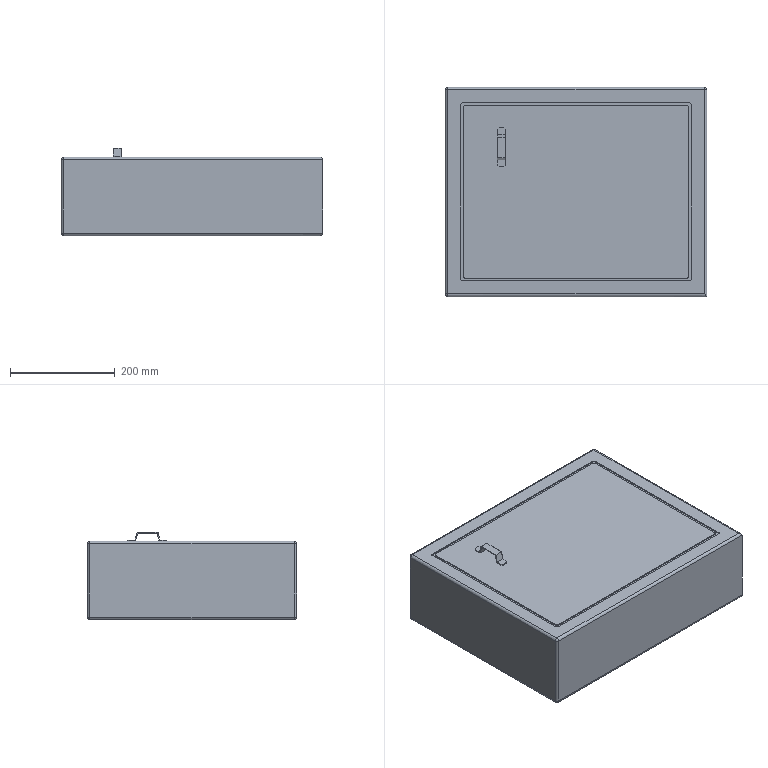Part | STEP file | electrical control box | 1 solid | 57 faces | box 500 x 400 x 167 mm | volume 29965916 mm3 | plane 32 | cylinder 19 | sphere 6 | commonest cylinder face diameters 10 x11 6 x8